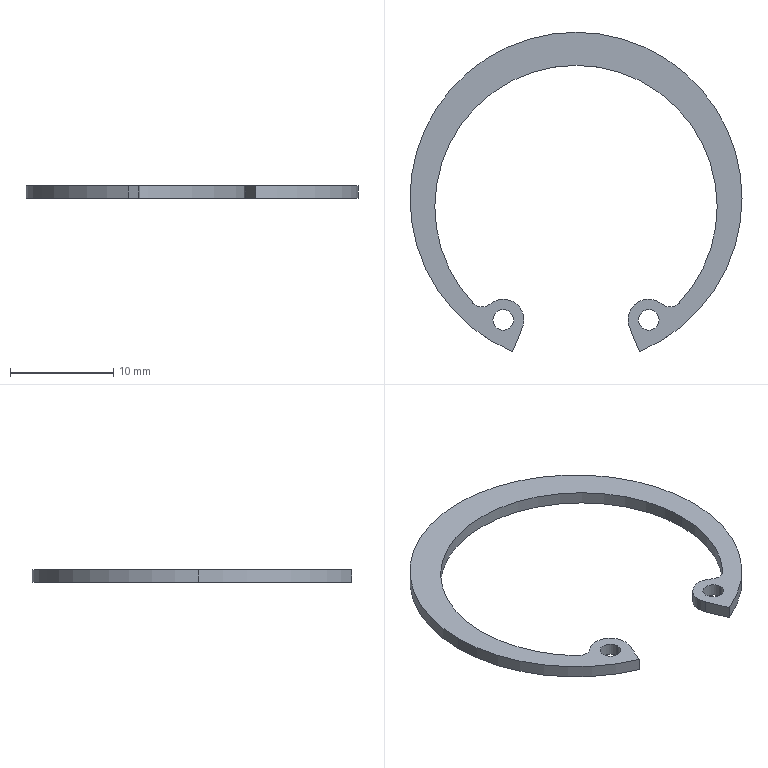Part | SolidWorks | features Extrusion 1 | 1 solid | 19 faces | box 32.1 x 30.878 x 1.2 mm | volume 259.483 mm3 | cylinder 15 | plane 4 | commonest cylinder face diameters 2 x4 4 x3 27.3 x3 32.1 x3 2.4 x2
STEP:
#1=CARTESIAN_POINT('',(-8.034,-11.756,-1.2));
#2=VERTEX_POINT('',#1);
#3=CARTESIAN_POINT('',(-6.034,-11.756,-1.2));
#4=VERTEX_POINT('',#3);
#5=CARTESIAN_POINT('',(-7.034,-11.756,-1.2));
#6=DIRECTION('',(0.,0.,1.));
#7=DIRECTION('',(1.,0.,0.));
#8=AXIS2_PLACEMENT_3D('',#5,#6,#7);
#9=CIRCLE('',#8,1.);
#10=EDGE_CURVE('',#2,#4,#9,.T.);
#11=ORIENTED_EDGE('',*,*,#10,.F.);
#12=CARTESIAN_POINT('',(-8.034,-11.756,0.));
#13=VERTEX_POINT('',#12);
#14=CARTESIAN_POINT('',(-8.034,-11.756,-1.2));
#15=DIRECTION('',(0.,0.,1.));
#16=VECTOR('',#15,1000.);
#17=LINE('',#14,#16);
#18=EDGE_CURVE('',#2,#13,#17,.T.);
#19=ORIENTED_EDGE('',*,*,#18,.T.);
#20=CARTESIAN_POINT('',(-6.034,-11.756,0.));
#21=VERTEX_POINT('',#20);
#22=CARTESIAN_POINT('',(-7.034,-11.756,0.));
#23=DIRECTION('',(0.,0.,1.));
#24=DIRECTION('',(1.,0.,0.));
#25=AXIS2_PLACEMENT_3D('',#22,#23,#24);
#26=CIRCLE('',#25,1.);
#27=EDGE_CURVE('',#13,#21,#26,.T.);
#28=ORIENTED_EDGE('',*,*,#27,.T.);
#29=CARTESIAN_POINT('',(-6.034,-11.756,-1.2));
#30=DIRECTION('',(0.,0.,1.));
#31=VECTOR('',#30,1000.);
#32=LINE('',#29,#31);
#33=EDGE_CURVE('',#4,#21,#32,.T.);
#34=ORIENTED_EDGE('',*,*,#33,.F.);
#35=EDGE_LOOP('',(#11,#19,#28,#34));
#36=FACE_OUTER_BOUND('',#35,.T.);
#37=CARTESIAN_POINT('',(-7.034,-11.756,-1.2));
#38=DIRECTION('',(0.,0.,1.));
#39=DIRECTION('',(1.,0.,0.));
#40=AXIS2_PLACEMENT_3D('',#37,#38,#39);
#41=CYLINDRICAL_SURFACE('',#40,1.);
#42=ADVANCED_FACE('',(#36),#41,.F.);
#43=CARTESIAN_POINT('',(6.034,-11.756,-1.2));
#44=VERTEX_POINT('',#43);
#45=CARTESIAN_POINT('',(8.034,-11.756,-1.2));
#46=VERTEX_POINT('',#45);
#47=CARTESIAN_POINT('',(7.034,-11.756,-1.2));
#48=DIRECTION('',(0.,0.,1.));
#49=DIRECTION('',(-1.,0.,0.));
#50=AXIS2_PLACEMENT_3D('',#47,#48,#49);
#51=CIRCLE('',#50,1.);
#52=EDGE_CURVE('',#44,#46,#51,.T.);
#53=ORIENTED_EDGE('',*,*,#52,.F.);
#54=CARTESIAN_POINT('',(6.034,-11.756,0.));
#55=VERTEX_POINT('',#54);
#56=CARTESIAN_POINT('',(6.034,-11.756,-1.2));
#57=DIRECTION('',(0.,0.,1.));
#58=VECTOR('',#57,1000.);
#59=LINE('',#56,#58);
#60=EDGE_CURVE('',#44,#55,#59,.T.);
#61=ORIENTED_EDGE('',*,*,#60,.T.);
#62=CARTESIAN_POINT('',(8.034,-11.756,0.));
#63=VERTEX_POINT('',#62);
#64=CARTESIAN_POINT('',(7.034,-11.756,0.));
#65=DIRECTION('',(0.,0.,1.));
#66=DIRECTION('',(-1.,0.,0.));
#67=AXIS2_PLACEMENT_3D('',#64,#65,#66);
#68=CIRCLE('',#67,1.);
#69=EDGE_CURVE('',#55,#63,#68,.T.);
#70=ORIENTED_EDGE('',*,*,#69,.T.);
#71=CARTESIAN_POINT('',(8.034,-11.756,-1.2));
#72=DIRECTION('',(0.,0.,1.));
#73=VECTOR('',#72,1000.);
#74=LINE('',#71,#73);
#75=EDGE_CURVE('',#46,#63,#74,.T.);
#76=ORIENTED_EDGE('',*,*,#75,.F.);
#77=EDGE_LOOP('',(#53,#61,#70,#76));
#78=FACE_OUTER_BOUND('',#77,.T.);
#79=CARTESIAN_POINT('',(7.034,-11.756,-1.2));
#80=DIRECTION('',(0.,0.,1.));
#81=DIRECTION('',(1.,0.,0.));
#82=AXIS2_PLACEMENT_3D('',#79,#80,#81);
#83=CYLINDRICAL_SURFACE('',#82,1.);
#84=ADVANCED_FACE('',(#78),#83,.F.);
#85=CARTESIAN_POINT('',(-5.187,-12.522,-1.2));
#86=VERTEX_POINT('',#85);
#87=CARTESIAN_POINT('',(-5.034,-11.756,-1.2));
#88=VERTEX_POINT('',#87);
#89=CARTESIAN_POINT('',(-7.034,-11.756,-1.2));
#90=DIRECTION('',(0.,0.,1.));
#91=DIRECTION('',(1.,0.,0.));
#92=AXIS2_PLACEMENT_3D('',#89,#90,#91);
#93=CIRCLE('',#92,2.);
#94=EDGE_CURVE('',#86,#88,#93,.T.);
#95=ORIENTED_EDGE('',*,*,#94,.T.);
#96=CARTESIAN_POINT('',(-5.034,-11.756,0.));
#97=VERTEX_POINT('',#96);
#98=CARTESIAN_POINT('',(-5.034,-11.756,-1.2));
#99=DIRECTION('',(0.,0.,1.));
#100=VECTOR('',#99,1000.);
#101=LINE('',#98,#100);
#102=EDGE_CURVE('',#88,#97,#101,.T.);
#103=ORIENTED_EDGE('',*,*,#102,.T.);
#104=CARTESIAN_POINT('',(-5.187,-12.522,0.));
#105=VERTEX_POINT('',#104);
#106=CARTESIAN_POINT('',(-7.034,-11.756,0.));
#107=DIRECTION('',(0.,0.,1.));
#108=DIRECTION('',(1.,0.,0.));
#109=AXIS2_PLACEMENT_3D('',#106,#107,#108);
#110=CIRCLE('',#109,2.);
#111=EDGE_CURVE('',#105,#97,#110,.T.);
#112=ORIENTED_EDGE('',*,*,#111,.F.);
#113=CARTESIAN_POINT('',(-5.187,-12.522,-1.2));
#114=DIRECTION('',(0.,0.,1.));
#115=VECTOR('',#114,1000.);
#116=LINE('',#113,#115);
#117=EDGE_CURVE('',#86,#105,#116,.T.);
#118=ORIENTED_EDGE('',*,*,#117,.F.);
#119=EDGE_LOOP('',(#95,#103,#112,#118));
#120=FACE_OUTER_BOUND('',#119,.T.);
#121=CARTESIAN_POINT('',(-7.034,-11.756,-1.2));
#122=DIRECTION('',(0.,0.,1.));
#123=DIRECTION('',(1.,0.,0.));
#124=AXIS2_PLACEMENT_3D('',#121,#122,#123);
#125=CYLINDRICAL_SURFACE('',#124,2.);
#126=ADVANCED_FACE('',(#120),#125,.T.);
#127=CARTESIAN_POINT('',(-9.968,-10.125,-1.2));
#128=VERTEX_POINT('',#127);
#129=CARTESIAN_POINT('',(-13.65,-0.8,-1.2));
#130=VERTEX_POINT('',#129);
#131=CARTESIAN_POINT('',(0.,-0.8,-1.2));
#132=DIRECTION('',(0.,0.,-1.));
#133=DIRECTION('',(1.,0.,0.));
#134=AXIS2_PLACEMENT_3D('',#131,#132,#133);
#135=CIRCLE('',#134,13.65);
#136=EDGE_CURVE('',#128,#130,#135,.T.);
#137=ORIENTED_EDGE('',*,*,#136,.T.);
#138=CARTESIAN_POINT('',(-13.65,-0.8,0.));
#139=VERTEX_POINT('',#138);
#140=CARTESIAN_POINT('',(-13.65,-0.8,-1.2));
#141=DIRECTION('',(0.,0.,1.));
#142=VECTOR('',#141,1000.);
#143=LINE('',#140,#142);
#144=EDGE_CURVE('',#130,#139,#143,.T.);
#145=ORIENTED_EDGE('',*,*,#144,.T.);
#146=CARTESIAN_POINT('',(-9.968,-10.125,0.));
#147=VERTEX_POINT('',#146);
#148=CARTESIAN_POINT('',(0.,-0.8,0.));
#149=DIRECTION('',(0.,0.,-1.));
#150=DIRECTION('',(1.,0.,0.));
#151=AXIS2_PLACEMENT_3D('',#148,#149,#150);
#152=CIRCLE('',#151,13.65);
#153=EDGE_CURVE('',#147,#139,#152,.T.);
#154=ORIENTED_EDGE('',*,*,#153,.F.);
#155=CARTESIAN_POINT('',(-9.968,-10.125,-1.2));
#156=DIRECTION('',(0.,0.,1.));
#157=VECTOR('',#156,1000.);
#158=LINE('',#155,#157);
#159=EDGE_CURVE('',#128,#147,#158,.T.);
#160=ORIENTED_EDGE('',*,*,#159,.F.);
#161=EDGE_LOOP('',(#137,#145,#154,#160));
#162=FACE_OUTER_BOUND('',#161,.T.);
#163=CARTESIAN_POINT('',(0.,-0.8,-1.2));
#164=DIRECTION('',(0.,0.,1.));
#165=DIRECTION('',(1.,0.,0.));
#166=AXIS2_PLACEMENT_3D('',#163,#164,#165);
#167=CYLINDRICAL_SURFACE('',#166,13.65);
#168=ADVANCED_FACE('',(#162),#167,.F.);
#169=ORIENTED_EDGE('',*,*,#144,.F.);
#170=CARTESIAN_POINT('',(13.65,-0.8,-1.2));
#171=VERTEX_POINT('',#170);
#172=CARTESIAN_POINT('',(0.,-0.8,-1.2));
#173=DIRECTION('',(0.,0.,-1.));
#174=DIRECTION('',(1.,0.,0.));
#175=AXIS2_PLACEMENT_3D('',#172,#173,#174);
#176=CIRCLE('',#175,13.65);
#177=EDGE_CURVE('',#130,#171,#176,.T.);
#178=ORIENTED_EDGE('',*,*,#177,.T.);
#179=CARTESIAN_POINT('',(13.65,-0.8,0.));
#180=VERTEX_POINT('',#179);
#181=CARTESIAN_POINT('',(13.65,-0.8,-1.2));
#182=DIRECTION('',(0.,0.,1.));
#183=VECTOR('',#182,1000.);
#184=LINE('',#181,#183);
#185=EDGE_CURVE('',#171,#180,#184,.T.);
#186=ORIENTED_EDGE('',*,*,#185,.T.);
#187=CARTESIAN_POINT('',(0.,-0.8,0.));
#188=DIRECTION('',(0.,0.,-1.));
#189=DIRECTION('',(1.,0.,0.));
#190=AXIS2_PLACEMENT_3D('',#187,#188,#189);
#191=CIRCLE('',#190,13.65);
#192=EDGE_CURVE('',#139,#180,#191,.T.);
#193=ORIENTED_EDGE('',*,*,#192,.F.);
#194=EDGE_LOOP('',(#169,#178,#186,#193));
#195=FACE_OUTER_BOUND('',#194,.T.);
#196=CARTESIAN_POINT('',(0.,-0.8,-1.2));
#197=DIRECTION('',(0.,0.,1.));
#198=DIRECTION('',(1.,0.,0.));
#199=AXIS2_PLACEMENT_3D('',#196,#197,#198);
#200=CYLINDRICAL_SURFACE('',#199,13.65);
#201=ADVANCED_FACE('',(#195),#200,.F.);
#202=CARTESIAN_POINT('',(16.05,0.,-1.2));
#203=VERTEX_POINT('',#202);
#204=CARTESIAN_POINT('',(-16.05,0.,-1.2));
#205=VERTEX_POINT('',#204);
#206=CARTESIAN_POINT('',(0.,0.,-1.2));
#207=DIRECTION('',(0.,0.,1.));
#208=DIRECTION('',(1.,0.,0.));
#209=AXIS2_PLACEMENT_3D('',#206,#207,#208);
#210=CIRCLE('',#209,16.05);
#211=EDGE_CURVE('',#203,#205,#210,.T.);
#212=ORIENTED_EDGE('',*,*,#211,.T.);
#213=CARTESIAN_POINT('',(-16.05,0.,0.));
#214=VERTEX_POINT('',#213);
#215=CARTESIAN_POINT('',(-16.05,0.,-1.2));
#216=DIRECTION('',(0.,0.,1.));
#217=VECTOR('',#216,1000.);
#218=LINE('',#215,#217);
#219=EDGE_CURVE('',#205,#214,#218,.T.);
#220=ORIENTED_EDGE('',*,*,#219,.T.);
#221=CARTESIAN_POINT('',(16.05,0.,0.));
#222=VERTEX_POINT('',#221);
#223=CARTESIAN_POINT('',(0.,0.,0.));
#224=DIRECTION('',(0.,0.,1.));
#225=DIRECTION('',(1.,0.,0.));
#226=AXIS2_PLACEMENT_3D('',#223,#224,#225);
#227=CIRCLE('',#226,16.05);
#228=EDGE_CURVE('',#222,#214,#227,.T.);
#229=ORIENTED_EDGE('',*,*,#228,.F.);
#230=CARTESIAN_POINT('',(16.05,0.,-1.2));
#231=DIRECTION('',(0.,0.,1.));
#232=VECTOR('',#231,1000.);
#233=LINE('',#230,#232);
#234=EDGE_CURVE('',#203,#222,#233,.T.);
#235=ORIENTED_EDGE('',*,*,#234,.F.);
#236=EDGE_LOOP('',(#212,#220,#229,#235));
#237=FACE_OUTER_BOUND('',#236,.T.);
#238=CARTESIAN_POINT('',(0.,0.,-1.2));
#239=DIRECTION('',(0.,0.,1.));
#240=DIRECTION('',(1.,0.,0.));
#241=AXIS2_PLACEMENT_3D('',#238,#239,#240);
#242=CYLINDRICAL_SURFACE('',#241,16.05);
#243=ADVANCED_FACE('',(#237),#242,.T.);
#244=CARTESIAN_POINT('',(6.142,-14.828,-1.2));
#245=VERTEX_POINT('',#244);
#246=CARTESIAN_POINT('',(0.,0.,-1.2));
#247=DIRECTION('',(0.,0.,1.));
#248=DIRECTION('',(1.,0.,0.));
#249=AXIS2_PLACEMENT_3D('',#246,#247,#248);
#250=CIRCLE('',#249,16.05);
#251=EDGE_CURVE('',#245,#203,#250,.T.);
#252=ORIENTED_EDGE('',*,*,#251,.T.);
#253=ORIENTED_EDGE('',*,*,#234,.T.);
#254=CARTESIAN_POINT('',(6.142,-14.828,0.));
#255=VERTEX_POINT('',#254);
#256=CARTESIAN_POINT('',(0.,0.,0.));
#257=DIRECTION('',(0.,0.,1.));
#258=DIRECTION('',(1.,0.,0.));
#259=AXIS2_PLACEMENT_3D('',#256,#257,#258);
#260=CIRCLE('',#259,16.05);
#261=EDGE_CURVE('',#255,#222,#260,.T.);
#262=ORIENTED_EDGE('',*,*,#261,.F.);
#263=CARTESIAN_POINT('',(6.142,-14.828,-1.2));
#264=DIRECTION('',(0.,0.,1.));
#265=VECTOR('',#264,1000.);
#266=LINE('',#263,#265);
#267=EDGE_CURVE('',#245,#255,#266,.T.);
#268=ORIENTED_EDGE('',*,*,#267,.F.);
#269=EDGE_LOOP('',(#252,#253,#262,#268));
#270=FACE_OUTER_BOUND('',#269,.T.);
#271=CARTESIAN_POINT('',(0.,0.,-1.2));
#272=DIRECTION('',(0.,0.,1.));
#273=DIRECTION('',(1.,0.,0.));
#274=AXIS2_PLACEMENT_3D('',#271,#272,#273);
#275=CYLINDRICAL_SURFACE('',#274,16.05);
#276=ADVANCED_FACE('',(#270),#275,.T.);
#277=ORIENTED_EDGE('',*,*,#219,.F.);
#278=CARTESIAN_POINT('',(-6.142,-14.828,-1.2));
#279=VERTEX_POINT('',#278);
#280=CARTESIAN_POINT('',(0.,0.,-1.2));
#281=DIRECTION('',(0.,0.,1.));
#282=DIRECTION('',(1.,0.,0.));
#283=AXIS2_PLACEMENT_3D('',#280,#281,#282);
#284=CIRCLE('',#283,16.05);
#285=EDGE_CURVE('',#205,#279,#284,.T.);
#286=ORIENTED_EDGE('',*,*,#285,.T.);
#287=CARTESIAN_POINT('',(-6.142,-14.828,0.));
#288=VERTEX_POINT('',#287);
#289=CARTESIAN_POINT('',(-6.142,-14.828,-1.2));
#290=DIRECTION('',(0.,0.,1.));
#291=VECTOR('',#290,1000.);
#292=LINE('',#289,#291);
#293=EDGE_CURVE('',#279,#288,#292,.T.);
#294=ORIENTED_EDGE('',*,*,#293,.T.);
#295=CARTESIAN_POINT('',(0.,0.,0.));
#296=DIRECTION('',(0.,0.,1.));
#297=DIRECTION('',(1.,0.,0.));
#298=AXIS2_PLACEMENT_3D('',#295,#296,#297);
#299=CIRCLE('',#298,16.05);
#300=EDGE_CURVE('',#214,#288,#299,.T.);
#301=ORIENTED_EDGE('',*,*,#300,.F.);
#302=EDGE_LOOP('',(#277,#286,#294,#301));
#303=FACE_OUTER_BOUND('',#302,.T.);
#304=CARTESIAN_POINT('',(0.,0.,-1.2));
#305=DIRECTION('',(0.,0.,1.));
#306=DIRECTION('',(1.,0.,0.));
#307=AXIS2_PLACEMENT_3D('',#304,#305,#306);
#308=CYLINDRICAL_SURFACE('',#307,16.05);
#309=ADVANCED_FACE('',(#303),#308,.T.);
#310=CARTESIAN_POINT('',(5.187,-12.522,0.));
#311=VERTEX_POINT('',#310);
#312=CARTESIAN_POINT('',(5.187,-12.522,0.));
#313=DIRECTION('',(0.3827,-0.9239,0.));
#314=VECTOR('',#313,1000.);
#315=LINE('',#312,#314);
#316=EDGE_CURVE('',#311,#255,#315,.T.);
#317=ORIENTED_EDGE('',*,*,#316,.F.);
#318=CARTESIAN_POINT('',(5.187,-12.522,-1.2));
#319=VERTEX_POINT('',#318);
#320=CARTESIAN_POINT('',(5.187,-12.522,-1.2));
#321=DIRECTION('',(0.,0.,1.));
#322=VECTOR('',#321,1000.);
#323=LINE('',#320,#322);
#324=EDGE_CURVE('',#319,#311,#323,.T.);
#325=ORIENTED_EDGE('',*,*,#324,.F.);
#326=CARTESIAN_POINT('',(5.187,-12.522,-1.2));
#327=DIRECTION('',(0.3827,-0.9239,0.));
#328=VECTOR('',#327,1000.);
#329=LINE('',#326,#328);
#330=EDGE_CURVE('',#319,#245,#329,.T.);
#331=ORIENTED_EDGE('',*,*,#330,.T.);
#332=ORIENTED_EDGE('',*,*,#267,.T.);
#333=EDGE_LOOP('',(#317,#325,#331,#332));
#334=FACE_OUTER_BOUND('',#333,.T.);
#335=CARTESIAN_POINT('',(5.187,-12.522,-1.2));
#336=DIRECTION('',(-0.9239,-0.3827,0.));
#337=DIRECTION('',(0.3827,-0.9239,0.));
#338=AXIS2_PLACEMENT_3D('',#335,#336,#337);
#339=PLANE('',#338);
#340=ADVANCED_FACE('',(#334),#339,.T.);
#341=CARTESIAN_POINT('',(8.32,-10.224,0.));
#342=VERTEX_POINT('',#341);
#343=CARTESIAN_POINT('',(7.034,-11.756,0.));
#344=DIRECTION('',(0.,0.,1.));
#345=DIRECTION('',(-1.,0.,0.));
#346=AXIS2_PLACEMENT_3D('',#343,#344,#345);
#347=CIRCLE('',#346,2.);
#348=EDGE_CURVE('',#342,#311,#347,.T.);
#349=ORIENTED_EDGE('',*,*,#348,.F.);
#350=CARTESIAN_POINT('',(8.32,-10.224,-1.2));
#351=VERTEX_POINT('',#350);
#352=CARTESIAN_POINT('',(8.32,-10.224,-1.2));
#353=DIRECTION('',(0.,0.,1.));
#354=VECTOR('',#353,1000.);
#355=LINE('',#352,#354);
#356=EDGE_CURVE('',#351,#342,#355,.T.);
#357=ORIENTED_EDGE('',*,*,#356,.F.);
#358=CARTESIAN_POINT('',(7.034,-11.756,-1.2));
#359=DIRECTION('',(0.,0.,1.));
#360=DIRECTION('',(-1.,0.,0.));
#361=AXIS2_PLACEMENT_3D('',#358,#359,#360);
#362=CIRCLE('',#361,2.);
#363=EDGE_CURVE('',#351,#319,#362,.T.);
#364=ORIENTED_EDGE('',*,*,#363,.T.);
#365=ORIENTED_EDGE('',*,*,#324,.T.);
#366=EDGE_LOOP('',(#349,#357,#364,#365));
#367=FACE_OUTER_BOUND('',#366,.T.);
#368=CARTESIAN_POINT('',(7.034,-11.756,-1.2));
#369=DIRECTION('',(0.,0.,1.));
#370=DIRECTION('',(1.,0.,0.));
#371=AXIS2_PLACEMENT_3D('',#368,#369,#370);
#372=CYLINDRICAL_SURFACE('',#371,2.);
#373=ADVANCED_FACE('',(#367),#372,.T.);
#374=CARTESIAN_POINT('',(9.968,-10.125,0.));
#375=VERTEX_POINT('',#374);
#376=CARTESIAN_POINT('',(9.092,-9.305,0.));
#377=DIRECTION('',(0.,0.,-1.));
#378=DIRECTION('',(-1.,0.,0.));
#379=AXIS2_PLACEMENT_3D('',#376,#377,#378);
#380=CIRCLE('',#379,1.2);
#381=EDGE_CURVE('',#375,#342,#380,.T.);
#382=ORIENTED_EDGE('',*,*,#381,.F.);
#383=CARTESIAN_POINT('',(9.968,-10.125,-1.2));
#384=VERTEX_POINT('',#383);
#385=CARTESIAN_POINT('',(9.968,-10.125,-1.2));
#386=DIRECTION('',(0.,0.,1.));
#387=VECTOR('',#386,1000.);
#388=LINE('',#385,#387);
#389=EDGE_CURVE('',#384,#375,#388,.T.);
#390=ORIENTED_EDGE('',*,*,#389,.F.);
#391=CARTESIAN_POINT('',(9.092,-9.305,-1.2));
#392=DIRECTION('',(0.,0.,-1.));
#393=DIRECTION('',(-1.,0.,0.));
#394=AXIS2_PLACEMENT_3D('',#391,#392,#393);
#395=CIRCLE('',#394,1.2);
#396=EDGE_CURVE('',#384,#351,#395,.T.);
#397=ORIENTED_EDGE('',*,*,#396,.T.);
#398=ORIENTED_EDGE('',*,*,#356,.T.);
#399=EDGE_LOOP('',(#382,#390,#397,#398));
#400=FACE_OUTER_BOUND('',#399,.T.);
#401=CARTESIAN_POINT('',(9.092,-9.305,-1.2));
#402=DIRECTION('',(0.,0.,1.));
#403=DIRECTION('',(1.,0.,0.));
#404=AXIS2_PLACEMENT_3D('',#401,#402,#403);
#405=CYLINDRICAL_SURFACE('',#404,1.2);
#406=ADVANCED_FACE('',(#400),#405,.F.);
#407=ORIENTED_EDGE('',*,*,#185,.F.);
#408=CARTESIAN_POINT('',(0.,-0.8,-1.2));
#409=DIRECTION('',(0.,0.,-1.));
#410=DIRECTION('',(1.,0.,0.));
#411=AXIS2_PLACEMENT_3D('',#408,#409,#410);
#412=CIRCLE('',#411,13.65);
#413=EDGE_CURVE('',#171,#384,#412,.T.);
#414=ORIENTED_EDGE('',*,*,#413,.T.);
#415=ORIENTED_EDGE('',*,*,#389,.T.);
#416=CARTESIAN_POINT('',(0.,-0.8,0.));
#417=DIRECTION('',(0.,0.,-1.));
#418=DIRECTION('',(1.,0.,0.));
#419=AXIS2_PLACEMENT_3D('',#416,#417,#418);
#420=CIRCLE('',#419,13.65);
#421=EDGE_CURVE('',#180,#375,#420,.T.);
#422=ORIENTED_EDGE('',*,*,#421,.F.);
#423=EDGE_LOOP('',(#407,#414,#415,#422));
#424=FACE_OUTER_BOUND('',#423,.T.);
#425=CARTESIAN_POINT('',(0.,-0.8,-1.2));
#426=DIRECTION('',(0.,0.,1.));
#427=DIRECTION('',(1.,0.,0.));
#428=AXIS2_PLACEMENT_3D('',#425,#426,#427);
#429=CYLINDRICAL_SURFACE('',#428,13.65);
#430=ADVANCED_FACE('',(#424),#429,.F.);
#431=CARTESIAN_POINT('',(-8.32,-10.224,0.));
#432=VERTEX_POINT('',#431);
#433=CARTESIAN_POINT('',(-9.092,-9.305,0.));
#434=DIRECTION('',(0.,0.,-1.));
#435=DIRECTION('',(1.,0.,0.));
#436=AXIS2_PLACEMENT_3D('',#433,#434,#435);
#437=CIRCLE('',#436,1.2);
#438=EDGE_CURVE('',#432,#147,#437,.T.);
#439=ORIENTED_EDGE('',*,*,#438,.F.);
#440=CARTESIAN_POINT('',(-8.32,-10.224,-1.2));
#441=VERTEX_POINT('',#440);
#442=CARTESIAN_POINT('',(-8.32,-10.224,-1.2));
#443=DIRECTION('',(0.,0.,1.));
#444=VECTOR('',#443,1000.);
#445=LINE('',#442,#444);
#446=EDGE_CURVE('',#441,#432,#445,.T.);
#447=ORIENTED_EDGE('',*,*,#446,.F.);
#448=CARTESIAN_POINT('',(-9.092,-9.305,-1.2));
#449=DIRECTION('',(0.,0.,-1.));
#450=DIRECTION('',(1.,0.,0.));
#451=AXIS2_PLACEMENT_3D('',#448,#449,#450);
#452=CIRCLE('',#451,1.2);
#453=EDGE_CURVE('',#441,#128,#452,.T.);
#454=ORIENTED_EDGE('',*,*,#453,.T.);
#455=ORIENTED_EDGE('',*,*,#159,.T.);
#456=EDGE_LOOP('',(#439,#447,#454,#455));
#457=FACE_OUTER_BOUND('',#456,.T.);
#458=CARTESIAN_POINT('',(-9.092,-9.305,-1.2));
#459=DIRECTION('',(0.,0.,1.));
#460=DIRECTION('',(1.,0.,0.));
#461=AXIS2_PLACEMENT_3D('',#458,#459,#460);
#462=CYLINDRICAL_SURFACE('',#461,1.2);
#463=ADVANCED_FACE('',(#457),#462,.F.);
#464=ORIENTED_EDGE('',*,*,#102,.F.);
#465=CARTESIAN_POINT('',(-7.034,-11.756,-1.2));
#466=DIRECTION('',(0.,0.,1.));
#467=DIRECTION('',(1.,0.,0.));
#468=AXIS2_PLACEMENT_3D('',#465,#466,#467);
#469=CIRCLE('',#468,2.);
#470=EDGE_CURVE('',#88,#441,#469,.T.);
#471=ORIENTED_EDGE('',*,*,#470,.T.);
#472=ORIENTED_EDGE('',*,*,#446,.T.);
#473=CARTESIAN_POINT('',(-7.034,-11.756,0.));
#474=DIRECTION('',(0.,0.,1.));
#475=DIRECTION('',(1.,0.,0.));
#476=AXIS2_PLACEMENT_3D('',#473,#474,#475);
#477=CIRCLE('',#476,2.);
#478=EDGE_CURVE('',#97,#432,#477,.T.);
#479=ORIENTED_EDGE('',*,*,#478,.F.);
#480=EDGE_LOOP('',(#464,#471,#472,#479));
#481=FACE_OUTER_BOUND('',#480,.T.);
#482=CARTESIAN_POINT('',(-7.034,-11.756,-1.2));
#483=DIRECTION('',(0.,0.,1.));
#484=DIRECTION('',(1.,0.,0.));
#485=AXIS2_PLACEMENT_3D('',#482,#483,#484);
#486=CYLINDRICAL_SURFACE('',#485,2.);
#487=ADVANCED_FACE('',(#481),#486,.T.);
#488=CARTESIAN_POINT('',(-5.187,-12.522,0.));
#489=DIRECTION('',(0.3827,0.9239,0.));
#490=VECTOR('',#489,1000.);
#491=LINE('',#488,#490);
#492=EDGE_CURVE('',#288,#105,#491,.T.);
#493=ORIENTED_EDGE('',*,*,#492,.F.);
#494=ORIENTED_EDGE('',*,*,#293,.F.);
#495=CARTESIAN_POINT('',(-5.187,-12.522,-1.2));
#496=DIRECTION('',(0.3827,0.9239,0.));
#497=VECTOR('',#496,1000.);
#498=LINE('',#495,#497);
#499=EDGE_CURVE('',#279,#86,#498,.T.);
#500=ORIENTED_EDGE('',*,*,#499,.T.);
#501=ORIENTED_EDGE('',*,*,#117,.T.);
#502=EDGE_LOOP('',(#493,#494,#500,#501));
#503=FACE_OUTER_BOUND('',#502,.T.);
#504=CARTESIAN_POINT('',(-5.187,-12.522,-1.2));
#505=DIRECTION('',(0.9239,-0.3827,0.));
#506=DIRECTION('',(0.3827,0.9239,0.));
#507=AXIS2_PLACEMENT_3D('',#504,#505,#506);
#508=PLANE('',#507);
#509=ADVANCED_FACE('',(#503),#508,.T.);
#510=CARTESIAN_POINT('',(-7.034,-11.756,-1.2));
#511=DIRECTION('',(0.,0.,1.));
#512=DIRECTION('',(1.,0.,0.));
#513=AXIS2_PLACEMENT_3D('',#510,#511,#512);
#514=CIRCLE('',#513,1.);
#515=EDGE_CURVE('',#4,#2,#514,.T.);
#516=ORIENTED_EDGE('',*,*,#515,.T.);
#517=ORIENTED_EDGE('',*,*,#10,.T.);
#518=EDGE_LOOP('',(#516,#517));
#519=FACE_BOUND('',#518,.T.);
#520=CARTESIAN_POINT('',(7.034,-11.756,-1.2));
#521=DIRECTION('',(0.,0.,1.));
#522=DIRECTION('',(-1.,0.,0.));
#523=AXIS2_PLACEMENT_3D('',#520,#521,#522);
#524=CIRCLE('',#523,1.);
#525=EDGE_CURVE('',#46,#44,#524,.T.);
#526=ORIENTED_EDGE('',*,*,#525,.T.);
#527=ORIENTED_EDGE('',*,*,#52,.T.);
#528=EDGE_LOOP('',(#526,#527));
#529=FACE_BOUND('',#528,.T.);
#530=ORIENTED_EDGE('',*,*,#251,.F.);
#531=ORIENTED_EDGE('',*,*,#330,.F.);
#532=ORIENTED_EDGE('',*,*,#363,.F.);
#533=ORIENTED_EDGE('',*,*,#396,.F.);
#534=ORIENTED_EDGE('',*,*,#413,.F.);
#535=ORIENTED_EDGE('',*,*,#177,.F.);
#536=ORIENTED_EDGE('',*,*,#136,.F.);
#537=ORIENTED_EDGE('',*,*,#453,.F.);
#538=ORIENTED_EDGE('',*,*,#470,.F.);
#539=ORIENTED_EDGE('',*,*,#94,.F.);
#540=ORIENTED_EDGE('',*,*,#499,.F.);
#541=ORIENTED_EDGE('',*,*,#285,.F.);
#542=ORIENTED_EDGE('',*,*,#211,.F.);
#543=EDGE_LOOP('',(#530,#531,#532,#533,#534,#535,#536,#537,#538,#539,#540,#541,#542));
#544=FACE_OUTER_BOUND('',#543,.T.);
#545=CARTESIAN_POINT('',(0.,0.,-1.2));
#546=DIRECTION('',(0.,0.,1.));
#547=DIRECTION('',(1.,0.,0.));
#548=AXIS2_PLACEMENT_3D('',#545,#546,#547);
#549=PLANE('',#548);
#550=ADVANCED_FACE('',(#519,#529,#544),#549,.F.);
#551=CARTESIAN_POINT('',(-7.034,-11.756,0.));
#552=DIRECTION('',(0.,0.,1.));
#553=DIRECTION('',(1.,0.,0.));
#554=AXIS2_PLACEMENT_3D('',#551,#552,#553);
#555=CIRCLE('',#554,1.);
#556=EDGE_CURVE('',#21,#13,#555,.T.);
#557=ORIENTED_EDGE('',*,*,#556,.F.);
#558=ORIENTED_EDGE('',*,*,#27,.F.);
#559=EDGE_LOOP('',(#557,#558));
#560=FACE_BOUND('',#559,.T.);
#561=CARTESIAN_POINT('',(7.034,-11.756,0.));
#562=DIRECTION('',(0.,0.,1.));
#563=DIRECTION('',(-1.,0.,0.));
#564=AXIS2_PLACEMENT_3D('',#561,#562,#563);
#565=CIRCLE('',#564,1.);
#566=EDGE_CURVE('',#63,#55,#565,.T.);
#567=ORIENTED_EDGE('',*,*,#566,.F.);
#568=ORIENTED_EDGE('',*,*,#69,.F.);
#569=EDGE_LOOP('',(#567,#568));
#570=FACE_BOUND('',#569,.T.);
#571=ORIENTED_EDGE('',*,*,#261,.T.);
#572=ORIENTED_EDGE('',*,*,#228,.T.);
#573=ORIENTED_EDGE('',*,*,#300,.T.);
#574=ORIENTED_EDGE('',*,*,#492,.T.);
#575=ORIENTED_EDGE('',*,*,#111,.T.);
#576=ORIENTED_EDGE('',*,*,#478,.T.);
#577=ORIENTED_EDGE('',*,*,#438,.T.);
#578=ORIENTED_EDGE('',*,*,#153,.T.);
#579=ORIENTED_EDGE('',*,*,#192,.T.);
#580=ORIENTED_EDGE('',*,*,#421,.T.);
#581=ORIENTED_EDGE('',*,*,#381,.T.);
#582=ORIENTED_EDGE('',*,*,#348,.T.);
#583=ORIENTED_EDGE('',*,*,#316,.T.);
#584=EDGE_LOOP('',(#571,#572,#573,#574,#575,#576,#577,#578,#579,#580,#581,#582,#583));
#585=FACE_OUTER_BOUND('',#584,.T.);
#586=CARTESIAN_POINT('',(0.,0.,0.));
#587=DIRECTION('',(0.,0.,1.));
#588=DIRECTION('',(1.,0.,0.));
#589=AXIS2_PLACEMENT_3D('',#586,#587,#588);
#590=PLANE('',#589);
#591=ADVANCED_FACE('',(#560,#570,#585),#590,.T.);
#592=ORIENTED_EDGE('',*,*,#60,.F.);
#593=ORIENTED_EDGE('',*,*,#525,.F.);
#594=ORIENTED_EDGE('',*,*,#75,.T.);
#595=ORIENTED_EDGE('',*,*,#566,.T.);
#596=EDGE_LOOP('',(#592,#593,#594,#595));
#597=FACE_OUTER_BOUND('',#596,.T.);
#598=CARTESIAN_POINT('',(7.034,-11.756,-1.2));
#599=DIRECTION('',(0.,0.,1.));
#600=DIRECTION('',(1.,0.,0.));
#601=AXIS2_PLACEMENT_3D('',#598,#599,#600);
#602=CYLINDRICAL_SURFACE('',#601,1.);
#603=ADVANCED_FACE('',(#597),#602,.F.);
#604=ORIENTED_EDGE('',*,*,#18,.F.);
#605=ORIENTED_EDGE('',*,*,#515,.F.);
#606=ORIENTED_EDGE('',*,*,#33,.T.);
#607=ORIENTED_EDGE('',*,*,#556,.T.);
#608=EDGE_LOOP('',(#604,#605,#606,#607));
#609=FACE_OUTER_BOUND('',#608,.T.);
#610=CARTESIAN_POINT('',(-7.034,-11.756,-1.2));
#611=DIRECTION('',(0.,0.,1.));
#612=DIRECTION('',(1.,0.,0.));
#613=AXIS2_PLACEMENT_3D('',#610,#611,#612);
#614=CYLINDRICAL_SURFACE('',#613,1.);
#615=ADVANCED_FACE('',(#609),#614,.F.);
#616=CLOSED_SHELL('',(#42,#84,#126,#168,#201,#243,#276,#309,#340,#373,#406,#430,#463,#487,#509,#550,#591,#603,#615));
#617=MANIFOLD_SOLID_BREP('',#616);
#618=CARTESIAN_POINT('',(0.,0.,0.));
#619=DIRECTION('',(0.,0.,1.));
#620=DIRECTION('',(1.,0.,0.));
#621=AXIS2_PLACEMENT_3D('',#618,#619,#620);
#622=(LENGTH_UNIT()NAMED_UNIT(*)SI_UNIT(.MILLI.,.METRE.));
#623=UNCERTAINTY_MEASURE_WITH_UNIT(LENGTH_MEASURE(0.00001),#622,'','');
#624=(NAMED_UNIT(*)PLANE_ANGLE_UNIT()SI_UNIT($,.RADIAN.));
#625=(NAMED_UNIT(*)SI_UNIT($,.STERADIAN.)SOLID_ANGLE_UNIT());
#626=(GEOMETRIC_REPRESENTATION_CONTEXT(3)GLOBAL_UNCERTAINTY_ASSIGNED_CONTEXT((#623))GLOBAL_UNIT_ASSIGNED_CONTEXT((#622,#624,#625))REPRESENTATION_CONTEXT('',''));
#627=ADVANCED_BREP_SHAPE_REPRESENTATION('',(#617,#621),#626);